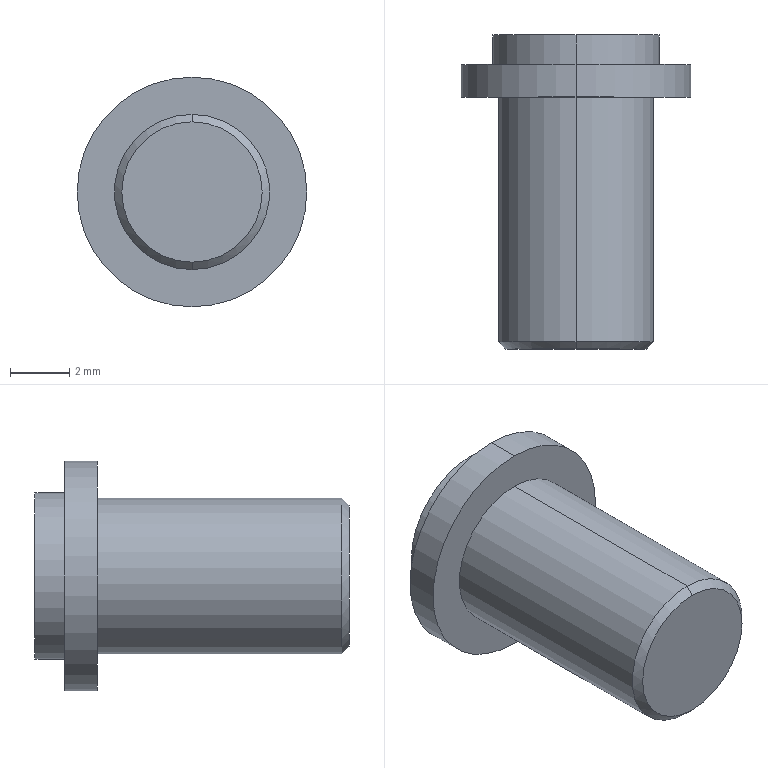Part | NX | features BREP 1 | 1 solid | 15 faces | box 7.75 x 10.6 x 7.75 mm | volume 133.839 mm3 | cylinder 8 | plane 5 | cone 2 | commonest cylinder face diameters 4 x2 5.24 x2 5.62 x2 7.75 x2
STEP:
#1=CARTESIAN_POINT('',(0.,0.25,2.62));
#2=VERTEX_POINT('',#1);
#3=CARTESIAN_POINT('',(0.,0.25,-2.62));
#4=VERTEX_POINT('',#3);
#5=CARTESIAN_POINT('',(0.,0.25,0.));
#6=DIRECTION('',(0.,1.,0.));
#7=DIRECTION('',(0.,0.,1.));
#8=AXIS2_PLACEMENT_3D('',#5,#6,#7);
#9=CIRCLE('',#8,2.62);
#10=EDGE_CURVE('',#2,#4,#9,.T.);
#11=ORIENTED_EDGE('',*,*,#10,.T.);
#12=CARTESIAN_POINT('',(0.,8.5,-2.62));
#13=VERTEX_POINT('',#12);
#14=CARTESIAN_POINT('',(0.,0.,-2.62));
#15=DIRECTION('',(0.,1.,0.));
#16=VECTOR('',#15,1000.);
#17=LINE('',#14,#16);
#18=EDGE_CURVE('',#4,#13,#17,.T.);
#19=ORIENTED_EDGE('',*,*,#18,.T.);
#20=CARTESIAN_POINT('',(0.,8.5,2.62));
#21=VERTEX_POINT('',#20);
#22=CARTESIAN_POINT('',(0.,8.5,0.));
#23=DIRECTION('',(0.,-1.,0.));
#24=DIRECTION('',(0.,0.,1.));
#25=AXIS2_PLACEMENT_3D('',#22,#23,#24);
#26=CIRCLE('',#25,2.62);
#27=EDGE_CURVE('',#13,#21,#26,.T.);
#28=ORIENTED_EDGE('',*,*,#27,.T.);
#29=CARTESIAN_POINT('',(0.,0.,2.62));
#30=DIRECTION('',(0.,1.,0.));
#31=VECTOR('',#30,1000.);
#32=LINE('',#29,#31);
#33=EDGE_CURVE('',#2,#21,#32,.T.);
#34=ORIENTED_EDGE('',*,*,#33,.F.);
#35=EDGE_LOOP('',(#11,#19,#28,#34));
#36=FACE_BOUND('',#35,.T.);
#37=CARTESIAN_POINT('',(0.,0.,0.));
#38=DIRECTION('',(0.,1.,0.));
#39=DIRECTION('',(0.,0.,-1.));
#40=AXIS2_PLACEMENT_3D('',#37,#38,#39);
#41=CYLINDRICAL_SURFACE('',#40,2.62);
#42=ADVANCED_FACE('',(#36),#41,.T.);
#43=CARTESIAN_POINT('',(0.,-0.000000306,2.37));
#44=VERTEX_POINT('',#43);
#45=CARTESIAN_POINT('',(0.,-0.000000306,-2.37));
#46=VERTEX_POINT('',#45);
#47=CARTESIAN_POINT('',(0.,-0.000000306,0.));
#48=DIRECTION('',(0.,1.,0.));
#49=DIRECTION('',(0.,0.,1.));
#50=AXIS2_PLACEMENT_3D('',#47,#48,#49);
#51=CIRCLE('',#50,2.37);
#52=EDGE_CURVE('',#44,#46,#51,.T.);
#53=ORIENTED_EDGE('',*,*,#52,.T.);
#54=CARTESIAN_POINT('',(0.,0.25,-2.62));
#55=DIRECTION('',(0.,0.7071,-0.7071));
#56=VECTOR('',#55,1000.);
#57=LINE('',#54,#56);
#58=EDGE_CURVE('',#46,#4,#57,.T.);
#59=ORIENTED_EDGE('',*,*,#58,.T.);
#60=ORIENTED_EDGE('',*,*,#10,.F.);
#61=CARTESIAN_POINT('',(0.,0.25,2.62));
#62=DIRECTION('',(0.,0.7071,0.7071));
#63=VECTOR('',#62,1000.);
#64=LINE('',#61,#63);
#65=EDGE_CURVE('',#44,#2,#64,.T.);
#66=ORIENTED_EDGE('',*,*,#65,.F.);
#67=EDGE_LOOP('',(#53,#59,#60,#66));
#68=FACE_BOUND('',#67,.T.);
#69=CARTESIAN_POINT('',(0.,0.25,0.));
#70=DIRECTION('',(0.,1.,0.));
#71=DIRECTION('',(0.,0.,-1.));
#72=AXIS2_PLACEMENT_3D('',#69,#70,#71);
#73=CONICAL_SURFACE('',#72,2.62,0.7854);
#74=ADVANCED_FACE('',(#68),#73,.T.);
#75=CARTESIAN_POINT('',(0.,8.5,3.875));
#76=VERTEX_POINT('',#75);
#77=CARTESIAN_POINT('',(0.,8.5,-3.875));
#78=VERTEX_POINT('',#77);
#79=CARTESIAN_POINT('',(0.,8.5,0.));
#80=DIRECTION('',(0.,1.,0.));
#81=DIRECTION('',(0.,0.,1.));
#82=AXIS2_PLACEMENT_3D('',#79,#80,#81);
#83=CIRCLE('',#82,3.875);
#84=EDGE_CURVE('',#76,#78,#83,.T.);
#85=ORIENTED_EDGE('',*,*,#84,.T.);
#86=CARTESIAN_POINT('',(0.,9.6,-3.875));
#87=VERTEX_POINT('',#86);
#88=CARTESIAN_POINT('',(0.,8.5,-3.875));
#89=DIRECTION('',(0.,1.,0.));
#90=VECTOR('',#89,1000.);
#91=LINE('',#88,#90);
#92=EDGE_CURVE('',#78,#87,#91,.T.);
#93=ORIENTED_EDGE('',*,*,#92,.T.);
#94=CARTESIAN_POINT('',(0.,9.6,3.875));
#95=VERTEX_POINT('',#94);
#96=CARTESIAN_POINT('',(0.,9.6,0.));
#97=DIRECTION('',(0.,-1.,0.));
#98=DIRECTION('',(0.,0.,1.));
#99=AXIS2_PLACEMENT_3D('',#96,#97,#98);
#100=CIRCLE('',#99,3.875);
#101=EDGE_CURVE('',#87,#95,#100,.T.);
#102=ORIENTED_EDGE('',*,*,#101,.T.);
#103=CARTESIAN_POINT('',(0.,8.5,3.875));
#104=DIRECTION('',(0.,1.,0.));
#105=VECTOR('',#104,1000.);
#106=LINE('',#103,#105);
#107=EDGE_CURVE('',#76,#95,#106,.T.);
#108=ORIENTED_EDGE('',*,*,#107,.F.);
#109=EDGE_LOOP('',(#85,#93,#102,#108));
#110=FACE_BOUND('',#109,.T.);
#111=CARTESIAN_POINT('',(0.,8.5,0.));
#112=DIRECTION('',(0.,1.,0.));
#113=DIRECTION('',(0.,0.,-1.));
#114=AXIS2_PLACEMENT_3D('',#111,#112,#113);
#115=CYLINDRICAL_SURFACE('',#114,3.875);
#116=ADVANCED_FACE('',(#110),#115,.T.);
#117=CARTESIAN_POINT('',(0.,9.6,-2.81));
#118=VERTEX_POINT('',#117);
#119=CARTESIAN_POINT('',(0.,9.6,2.81));
#120=VERTEX_POINT('',#119);
#121=CARTESIAN_POINT('',(0.,9.6,0.));
#122=DIRECTION('',(0.,-1.,0.));
#123=DIRECTION('',(0.,0.,1.));
#124=AXIS2_PLACEMENT_3D('',#121,#122,#123);
#125=CIRCLE('',#124,2.81);
#126=EDGE_CURVE('',#118,#120,#125,.T.);
#127=ORIENTED_EDGE('',*,*,#126,.F.);
#128=CARTESIAN_POINT('',(0.,10.6,-2.81));
#129=VERTEX_POINT('',#128);
#130=CARTESIAN_POINT('',(0.,9.6,-2.81));
#131=DIRECTION('',(0.,1.,0.));
#132=VECTOR('',#131,1000.);
#133=LINE('',#130,#132);
#134=EDGE_CURVE('',#118,#129,#133,.T.);
#135=ORIENTED_EDGE('',*,*,#134,.T.);
#136=CARTESIAN_POINT('',(0.,10.6,2.81));
#137=VERTEX_POINT('',#136);
#138=CARTESIAN_POINT('',(0.,10.6,0.));
#139=DIRECTION('',(0.,-1.,0.));
#140=DIRECTION('',(0.,0.,1.));
#141=AXIS2_PLACEMENT_3D('',#138,#139,#140);
#142=CIRCLE('',#141,2.81);
#143=EDGE_CURVE('',#129,#137,#142,.T.);
#144=ORIENTED_EDGE('',*,*,#143,.T.);
#145=CARTESIAN_POINT('',(0.,9.6,2.81));
#146=DIRECTION('',(0.,1.,0.));
#147=VECTOR('',#146,1000.);
#148=LINE('',#145,#147);
#149=EDGE_CURVE('',#120,#137,#148,.T.);
#150=ORIENTED_EDGE('',*,*,#149,.F.);
#151=EDGE_LOOP('',(#127,#135,#144,#150));
#152=FACE_BOUND('',#151,.T.);
#153=CARTESIAN_POINT('',(0.,9.6,0.));
#154=DIRECTION('',(0.,1.,0.));
#155=DIRECTION('',(0.,0.,-1.));
#156=AXIS2_PLACEMENT_3D('',#153,#154,#155);
#157=CYLINDRICAL_SURFACE('',#156,2.81);
#158=ADVANCED_FACE('',(#152),#157,.T.);
#159=CARTESIAN_POINT('',(0.,0.6,-2.));
#160=VERTEX_POINT('',#159);
#161=CARTESIAN_POINT('',(0.,0.6,2.));
#162=VERTEX_POINT('',#161);
#163=CARTESIAN_POINT('',(0.,0.6,0.));
#164=DIRECTION('',(0.,1.,0.));
#165=DIRECTION('',(0.,0.,1.));
#166=AXIS2_PLACEMENT_3D('',#163,#164,#165);
#167=CIRCLE('',#166,2.);
#168=EDGE_CURVE('',#160,#162,#167,.T.);
#169=ORIENTED_EDGE('',*,*,#168,.F.);
#170=CARTESIAN_POINT('',(0.,10.6,-2.));
#171=VERTEX_POINT('',#170);
#172=CARTESIAN_POINT('',(0.,10.6,-2.));
#173=DIRECTION('',(0.,1.,0.));
#174=VECTOR('',#173,1000.);
#175=LINE('',#172,#174);
#176=EDGE_CURVE('',#160,#171,#175,.T.);
#177=ORIENTED_EDGE('',*,*,#176,.T.);
#178=CARTESIAN_POINT('',(0.,10.6,2.));
#179=VERTEX_POINT('',#178);
#180=CARTESIAN_POINT('',(0.,10.6,0.));
#181=DIRECTION('',(0.,-1.,0.));
#182=DIRECTION('',(0.,0.,1.));
#183=AXIS2_PLACEMENT_3D('',#180,#181,#182);
#184=CIRCLE('',#183,2.);
#185=EDGE_CURVE('',#179,#171,#184,.T.);
#186=ORIENTED_EDGE('',*,*,#185,.F.);
#187=CARTESIAN_POINT('',(0.,10.6,2.));
#188=DIRECTION('',(0.,1.,0.));
#189=VECTOR('',#188,1000.);
#190=LINE('',#187,#189);
#191=EDGE_CURVE('',#162,#179,#190,.T.);
#192=ORIENTED_EDGE('',*,*,#191,.F.);
#193=EDGE_LOOP('',(#169,#177,#186,#192));
#194=FACE_BOUND('',#193,.T.);
#195=CARTESIAN_POINT('',(0.,10.6,0.));
#196=DIRECTION('',(0.,1.,0.));
#197=DIRECTION('',(0.,0.,-1.));
#198=AXIS2_PLACEMENT_3D('',#195,#196,#197);
#199=CYLINDRICAL_SURFACE('',#198,2.);
#200=ADVANCED_FACE('',(#194),#199,.F.);
#201=ORIENTED_EDGE('',*,*,#18,.F.);
#202=CARTESIAN_POINT('',(0.,0.25,0.));
#203=DIRECTION('',(0.,1.,0.));
#204=DIRECTION('',(0.,0.,1.));
#205=AXIS2_PLACEMENT_3D('',#202,#203,#204);
#206=CIRCLE('',#205,2.62);
#207=EDGE_CURVE('',#4,#2,#206,.T.);
#208=ORIENTED_EDGE('',*,*,#207,.T.);
#209=ORIENTED_EDGE('',*,*,#33,.T.);
#210=CARTESIAN_POINT('',(0.,8.5,0.));
#211=DIRECTION('',(0.,-1.,0.));
#212=DIRECTION('',(0.,0.,1.));
#213=AXIS2_PLACEMENT_3D('',#210,#211,#212);
#214=CIRCLE('',#213,2.62);
#215=EDGE_CURVE('',#21,#13,#214,.T.);
#216=ORIENTED_EDGE('',*,*,#215,.T.);
#217=EDGE_LOOP('',(#201,#208,#209,#216));
#218=FACE_BOUND('',#217,.T.);
#219=CARTESIAN_POINT('',(0.,0.,0.));
#220=DIRECTION('',(0.,1.,0.));
#221=DIRECTION('',(0.,0.,-1.));
#222=AXIS2_PLACEMENT_3D('',#219,#220,#221);
#223=CYLINDRICAL_SURFACE('',#222,2.62);
#224=ADVANCED_FACE('',(#218),#223,.T.);
#225=ORIENTED_EDGE('',*,*,#84,.F.);
#226=CARTESIAN_POINT('',(0.,8.5,0.));
#227=DIRECTION('',(0.,1.,0.));
#228=DIRECTION('',(0.,0.,1.));
#229=AXIS2_PLACEMENT_3D('',#226,#227,#228);
#230=CIRCLE('',#229,3.875);
#231=EDGE_CURVE('',#78,#76,#230,.T.);
#232=ORIENTED_EDGE('',*,*,#231,.F.);
#233=EDGE_LOOP('',(#225,#232));
#234=FACE_BOUND('',#233,.T.);
#235=ORIENTED_EDGE('',*,*,#215,.F.);
#236=ORIENTED_EDGE('',*,*,#27,.F.);
#237=EDGE_LOOP('',(#235,#236));
#238=FACE_BOUND('',#237,.T.);
#239=CARTESIAN_POINT('',(0.,8.5,0.));
#240=DIRECTION('',(0.,1.,0.));
#241=DIRECTION('',(0.,0.,-1.));
#242=AXIS2_PLACEMENT_3D('',#239,#240,#241);
#243=PLANE('',#242);
#244=ADVANCED_FACE('',(#234,#238),#243,.F.);
#245=ORIENTED_EDGE('',*,*,#58,.F.);
#246=CARTESIAN_POINT('',(0.,-0.000000306,0.));
#247=DIRECTION('',(0.,1.,0.));
#248=DIRECTION('',(0.,0.,1.));
#249=AXIS2_PLACEMENT_3D('',#246,#247,#248);
#250=CIRCLE('',#249,2.37);
#251=EDGE_CURVE('',#46,#44,#250,.T.);
#252=ORIENTED_EDGE('',*,*,#251,.T.);
#253=ORIENTED_EDGE('',*,*,#65,.T.);
#254=ORIENTED_EDGE('',*,*,#207,.F.);
#255=EDGE_LOOP('',(#245,#252,#253,#254));
#256=FACE_BOUND('',#255,.T.);
#257=CARTESIAN_POINT('',(0.,0.25,0.));
#258=DIRECTION('',(0.,1.,0.));
#259=DIRECTION('',(0.,0.,-1.));
#260=AXIS2_PLACEMENT_3D('',#257,#258,#259);
#261=CONICAL_SURFACE('',#260,2.62,0.7854);
#262=ADVANCED_FACE('',(#256),#261,.T.);
#263=ORIENTED_EDGE('',*,*,#92,.F.);
#264=ORIENTED_EDGE('',*,*,#231,.T.);
#265=ORIENTED_EDGE('',*,*,#107,.T.);
#266=CARTESIAN_POINT('',(0.,9.6,0.));
#267=DIRECTION('',(0.,-1.,0.));
#268=DIRECTION('',(0.,0.,1.));
#269=AXIS2_PLACEMENT_3D('',#266,#267,#268);
#270=CIRCLE('',#269,3.875);
#271=EDGE_CURVE('',#95,#87,#270,.T.);
#272=ORIENTED_EDGE('',*,*,#271,.T.);
#273=EDGE_LOOP('',(#263,#264,#265,#272));
#274=FACE_BOUND('',#273,.T.);
#275=CARTESIAN_POINT('',(0.,8.5,0.));
#276=DIRECTION('',(0.,1.,0.));
#277=DIRECTION('',(0.,0.,-1.));
#278=AXIS2_PLACEMENT_3D('',#275,#276,#277);
#279=CYLINDRICAL_SURFACE('',#278,3.875);
#280=ADVANCED_FACE('',(#274),#279,.T.);
#281=ORIENTED_EDGE('',*,*,#52,.F.);
#282=ORIENTED_EDGE('',*,*,#251,.F.);
#283=EDGE_LOOP('',(#281,#282));
#284=FACE_BOUND('',#283,.T.);
#285=CARTESIAN_POINT('',(0.,0.,0.));
#286=DIRECTION('',(0.,1.,0.));
#287=DIRECTION('',(0.,0.,-1.));
#288=AXIS2_PLACEMENT_3D('',#285,#286,#287);
#289=PLANE('',#288);
#290=ADVANCED_FACE('',(#284),#289,.F.);
#291=ORIENTED_EDGE('',*,*,#271,.F.);
#292=ORIENTED_EDGE('',*,*,#101,.F.);
#293=EDGE_LOOP('',(#291,#292));
#294=FACE_BOUND('',#293,.T.);
#295=CARTESIAN_POINT('',(0.,9.6,0.));
#296=DIRECTION('',(0.,-1.,0.));
#297=DIRECTION('',(0.,0.,1.));
#298=AXIS2_PLACEMENT_3D('',#295,#296,#297);
#299=CIRCLE('',#298,2.81);
#300=EDGE_CURVE('',#120,#118,#299,.T.);
#301=ORIENTED_EDGE('',*,*,#300,.T.);
#302=ORIENTED_EDGE('',*,*,#126,.T.);
#303=EDGE_LOOP('',(#301,#302));
#304=FACE_BOUND('',#303,.T.);
#305=CARTESIAN_POINT('',(0.,9.6,0.));
#306=DIRECTION('',(0.,1.,0.));
#307=DIRECTION('',(0.,0.,-1.));
#308=AXIS2_PLACEMENT_3D('',#305,#306,#307);
#309=PLANE('',#308);
#310=ADVANCED_FACE('',(#294,#304),#309,.T.);
#311=ORIENTED_EDGE('',*,*,#134,.F.);
#312=ORIENTED_EDGE('',*,*,#300,.F.);
#313=ORIENTED_EDGE('',*,*,#149,.T.);
#314=CARTESIAN_POINT('',(0.,10.6,0.));
#315=DIRECTION('',(0.,-1.,0.));
#316=DIRECTION('',(0.,0.,1.));
#317=AXIS2_PLACEMENT_3D('',#314,#315,#316);
#318=CIRCLE('',#317,2.81);
#319=EDGE_CURVE('',#137,#129,#318,.T.);
#320=ORIENTED_EDGE('',*,*,#319,.T.);
#321=EDGE_LOOP('',(#311,#312,#313,#320));
#322=FACE_BOUND('',#321,.T.);
#323=CARTESIAN_POINT('',(0.,9.6,0.));
#324=DIRECTION('',(0.,1.,0.));
#325=DIRECTION('',(0.,0.,-1.));
#326=AXIS2_PLACEMENT_3D('',#323,#324,#325);
#327=CYLINDRICAL_SURFACE('',#326,2.81);
#328=ADVANCED_FACE('',(#322),#327,.T.);
#329=ORIENTED_EDGE('',*,*,#319,.F.);
#330=ORIENTED_EDGE('',*,*,#143,.F.);
#331=EDGE_LOOP('',(#329,#330));
#332=FACE_BOUND('',#331,.T.);
#333=ORIENTED_EDGE('',*,*,#185,.T.);
#334=CARTESIAN_POINT('',(0.,10.6,0.));
#335=DIRECTION('',(0.,-1.,0.));
#336=DIRECTION('',(0.,0.,1.));
#337=AXIS2_PLACEMENT_3D('',#334,#335,#336);
#338=CIRCLE('',#337,2.);
#339=EDGE_CURVE('',#171,#179,#338,.T.);
#340=ORIENTED_EDGE('',*,*,#339,.T.);
#341=EDGE_LOOP('',(#333,#340));
#342=FACE_BOUND('',#341,.T.);
#343=CARTESIAN_POINT('',(0.,10.6,0.));
#344=DIRECTION('',(0.,1.,0.));
#345=DIRECTION('',(0.,0.,-1.));
#346=AXIS2_PLACEMENT_3D('',#343,#344,#345);
#347=PLANE('',#346);
#348=ADVANCED_FACE('',(#332,#342),#347,.T.);
#349=ORIENTED_EDGE('',*,*,#176,.F.);
#350=CARTESIAN_POINT('',(0.,0.6,0.));
#351=DIRECTION('',(0.,1.,0.));
#352=DIRECTION('',(0.,0.,1.));
#353=AXIS2_PLACEMENT_3D('',#350,#351,#352);
#354=CIRCLE('',#353,2.);
#355=EDGE_CURVE('',#162,#160,#354,.T.);
#356=ORIENTED_EDGE('',*,*,#355,.F.);
#357=ORIENTED_EDGE('',*,*,#191,.T.);
#358=ORIENTED_EDGE('',*,*,#339,.F.);
#359=EDGE_LOOP('',(#349,#356,#357,#358));
#360=FACE_BOUND('',#359,.T.);
#361=CARTESIAN_POINT('',(0.,10.6,0.));
#362=DIRECTION('',(0.,1.,0.));
#363=DIRECTION('',(0.,0.,-1.));
#364=AXIS2_PLACEMENT_3D('',#361,#362,#363);
#365=CYLINDRICAL_SURFACE('',#364,2.);
#366=ADVANCED_FACE('',(#360),#365,.F.);
#367=ORIENTED_EDGE('',*,*,#355,.T.);
#368=ORIENTED_EDGE('',*,*,#168,.T.);
#369=EDGE_LOOP('',(#367,#368));
#370=FACE_BOUND('',#369,.T.);
#371=CARTESIAN_POINT('',(0.,0.6,0.));
#372=DIRECTION('',(0.,1.,0.));
#373=DIRECTION('',(0.,0.,-1.));
#374=AXIS2_PLACEMENT_3D('',#371,#372,#373);
#375=PLANE('',#374);
#376=ADVANCED_FACE('',(#370),#375,.T.);
#377=CLOSED_SHELL('',(#42,#74,#116,#158,#200,#224,#244,#262,#280,#290,#310,#328,#348,#366,#376));
#378=MANIFOLD_SOLID_BREP('',#377);
#379=(LENGTH_UNIT()NAMED_UNIT(*)SI_UNIT(.MILLI.,.METRE.));
#380=UNCERTAINTY_MEASURE_WITH_UNIT(LENGTH_MEASURE(0.00001),#379,'','');
#381=(NAMED_UNIT(*)PLANE_ANGLE_UNIT()SI_UNIT($,.RADIAN.));
#382=(NAMED_UNIT(*)SI_UNIT($,.STERADIAN.)SOLID_ANGLE_UNIT());
#383=(GEOMETRIC_REPRESENTATION_CONTEXT(3)GLOBAL_UNCERTAINTY_ASSIGNED_CONTEXT((#380))GLOBAL_UNIT_ASSIGNED_CONTEXT((#379,#381,#382))REPRESENTATION_CONTEXT('',''));
#384=ADVANCED_BREP_SHAPE_REPRESENTATION('',(#378),#383);